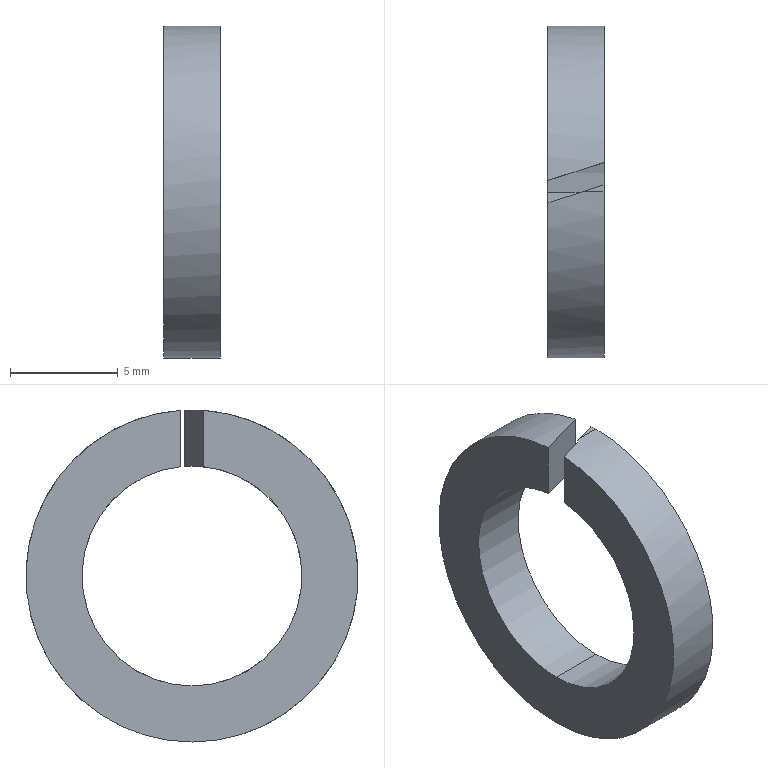Part | SolidWorks | features BaseBody 1 | 1 solid | 10 faces | box 2.6 x 15.4 x 15.4 mm | volume 264.776 mm3 | cylinder 6 | plane 4 | commonest cylinder face diameters 10.2 x3 15.4 x3
STEP:
#1=CARTESIAN_POINT('',(2.6,0.3248,7.693));
#2=VERTEX_POINT('',#1);
#3=CARTESIAN_POINT('',(1.6,0.,7.7));
#4=VERTEX_POINT('',#3);
#5=CARTESIAN_POINT('',(2.6,0.3248,7.693));
#6=CARTESIAN_POINT('',(2.267,0.2166,7.698));
#7=CARTESIAN_POINT('',(1.934,0.1083,7.7));
#8=CARTESIAN_POINT('',(1.6,0.,7.7));
#9=(BOUNDED_CURVE()B_SPLINE_CURVE(3,(#5,#6,#7,#8),.UNSPECIFIED.,.F.,.F.)B_SPLINE_CURVE_WITH_KNOTS((4,4),(1.529,1.571),.UNSPECIFIED.)CURVE()GEOMETRIC_REPRESENTATION_ITEM()RATIONAL_B_SPLINE_CURVE((1.,0.9999,0.9999,1.))REPRESENTATION_ITEM(''));
#10=EDGE_CURVE('',#2,#4,#9,.T.);
#11=ORIENTED_EDGE('',*,*,#10,.T.);
#12=CARTESIAN_POINT('',(2.6,0.,7.7));
#13=VERTEX_POINT('',#12);
#14=CARTESIAN_POINT('',(0.,0.,7.7));
#15=DIRECTION('',(1.,0.,0.));
#16=VECTOR('',#15,1000.);
#17=LINE('',#14,#16);
#18=EDGE_CURVE('',#4,#13,#17,.T.);
#19=ORIENTED_EDGE('',*,*,#18,.T.);
#20=CARTESIAN_POINT('',(2.6,0.,0.));
#21=DIRECTION('',(-1.,0.,0.));
#22=DIRECTION('',(0.,0.,-1.));
#23=AXIS2_PLACEMENT_3D('',#20,#21,#22);
#24=CIRCLE('',#23,7.7);
#25=EDGE_CURVE('',#13,#2,#24,.T.);
#26=ORIENTED_EDGE('',*,*,#25,.T.);
#27=EDGE_LOOP('',(#11,#19,#26));
#28=FACE_OUTER_BOUND('',#27,.T.);
#29=CARTESIAN_POINT('',(0.,0.,0.));
#30=DIRECTION('',(1.,0.,0.));
#31=DIRECTION('',(0.,0.,-1.));
#32=AXIS2_PLACEMENT_3D('',#29,#30,#31);
#33=CYLINDRICAL_SURFACE('',#32,7.7);
#34=ADVANCED_FACE('',(#28),#33,.T.);
#35=ORIENTED_EDGE('',*,*,#18,.F.);
#36=CARTESIAN_POINT('',(0.,-0.52,7.682));
#37=VERTEX_POINT('',#36);
#38=CARTESIAN_POINT('',(1.6,0.,7.7));
#39=CARTESIAN_POINT('',(1.066,-0.1735,7.7));
#40=CARTESIAN_POINT('',(0.5328,-0.3469,7.694));
#41=CARTESIAN_POINT('',(0.,-0.52,7.682));
#42=(BOUNDED_CURVE()B_SPLINE_CURVE(3,(#38,#39,#40,#41),.UNSPECIFIED.,.F.,.F.)B_SPLINE_CURVE_WITH_KNOTS((4,4),(1.571,1.638),.UNSPECIFIED.)CURVE()GEOMETRIC_REPRESENTATION_ITEM()RATIONAL_B_SPLINE_CURVE((1.,0.9996,0.9996,1.))REPRESENTATION_ITEM(''));
#43=EDGE_CURVE('',#4,#37,#42,.T.);
#44=ORIENTED_EDGE('',*,*,#43,.T.);
#45=CARTESIAN_POINT('',(0.,0.,-7.7));
#46=VERTEX_POINT('',#45);
#47=CARTESIAN_POINT('',(0.,0.,0.));
#48=DIRECTION('',(1.,0.,0.));
#49=DIRECTION('',(0.,0.,-1.));
#50=AXIS2_PLACEMENT_3D('',#47,#48,#49);
#51=CIRCLE('',#50,7.7);
#52=EDGE_CURVE('',#37,#46,#51,.T.);
#53=ORIENTED_EDGE('',*,*,#52,.T.);
#54=CARTESIAN_POINT('',(2.6,0.,-7.7));
#55=VERTEX_POINT('',#54);
#56=CARTESIAN_POINT('',(0.,0.,-7.7));
#57=DIRECTION('',(1.,0.,0.));
#58=VECTOR('',#57,1000.);
#59=LINE('',#56,#58);
#60=EDGE_CURVE('',#46,#55,#59,.T.);
#61=ORIENTED_EDGE('',*,*,#60,.T.);
#62=CARTESIAN_POINT('',(2.6,0.,0.));
#63=DIRECTION('',(-1.,0.,0.));
#64=DIRECTION('',(0.,0.,-1.));
#65=AXIS2_PLACEMENT_3D('',#62,#63,#64);
#66=CIRCLE('',#65,7.7);
#67=EDGE_CURVE('',#55,#13,#66,.T.);
#68=ORIENTED_EDGE('',*,*,#67,.T.);
#69=EDGE_LOOP('',(#35,#44,#53,#61,#68));
#70=FACE_OUTER_BOUND('',#69,.T.);
#71=CARTESIAN_POINT('',(0.,0.,0.));
#72=DIRECTION('',(1.,0.,0.));
#73=DIRECTION('',(0.,0.,-1.));
#74=AXIS2_PLACEMENT_3D('',#71,#72,#73);
#75=CYLINDRICAL_SURFACE('',#74,7.7);
#76=ADVANCED_FACE('',(#70),#75,.T.);
#77=CARTESIAN_POINT('',(0.,-0.52,5.073));
#78=VERTEX_POINT('',#77);
#79=CARTESIAN_POINT('',(1.6,0.,5.1));
#80=VERTEX_POINT('',#79);
#81=CARTESIAN_POINT('',(0.,-0.52,5.073));
#82=CARTESIAN_POINT('',(0.5318,-0.3472,5.091));
#83=CARTESIAN_POINT('',(1.066,-0.1737,5.1));
#84=CARTESIAN_POINT('',(1.6,0.,5.1));
#85=(BOUNDED_CURVE()B_SPLINE_CURVE(3,(#81,#82,#83,#84),.UNSPECIFIED.,.F.,.F.)B_SPLINE_CURVE_WITH_KNOTS((4,4),(4.61,4.712),.UNSPECIFIED.)CURVE()GEOMETRIC_REPRESENTATION_ITEM()RATIONAL_B_SPLINE_CURVE((1.,0.9991,0.9991,1.))REPRESENTATION_ITEM(''));
#86=EDGE_CURVE('',#78,#80,#85,.T.);
#87=ORIENTED_EDGE('',*,*,#86,.T.);
#88=CARTESIAN_POINT('',(2.6,0.,5.1));
#89=VERTEX_POINT('',#88);
#90=CARTESIAN_POINT('',(0.,0.,5.1));
#91=DIRECTION('',(1.,0.,0.));
#92=VECTOR('',#91,1000.);
#93=LINE('',#90,#92);
#94=EDGE_CURVE('',#80,#89,#93,.T.);
#95=ORIENTED_EDGE('',*,*,#94,.T.);
#96=CARTESIAN_POINT('',(2.6,0.,-5.1));
#97=VERTEX_POINT('',#96);
#98=CARTESIAN_POINT('',(2.6,0.,0.));
#99=DIRECTION('',(1.,0.,0.));
#100=DIRECTION('',(0.,0.,-1.));
#101=AXIS2_PLACEMENT_3D('',#98,#99,#100);
#102=CIRCLE('',#101,5.1);
#103=EDGE_CURVE('',#89,#97,#102,.T.);
#104=ORIENTED_EDGE('',*,*,#103,.T.);
#105=CARTESIAN_POINT('',(0.,0.,-5.1));
#106=VERTEX_POINT('',#105);
#107=CARTESIAN_POINT('',(0.,0.,-5.1));
#108=DIRECTION('',(1.,0.,0.));
#109=VECTOR('',#108,1000.);
#110=LINE('',#107,#109);
#111=EDGE_CURVE('',#106,#97,#110,.T.);
#112=ORIENTED_EDGE('',*,*,#111,.F.);
#113=CARTESIAN_POINT('',(0.,0.,0.));
#114=DIRECTION('',(1.,0.,0.));
#115=DIRECTION('',(0.,0.,-1.));
#116=AXIS2_PLACEMENT_3D('',#113,#114,#115);
#117=CIRCLE('',#116,5.1);
#118=EDGE_CURVE('',#78,#106,#117,.T.);
#119=ORIENTED_EDGE('',*,*,#118,.F.);
#120=EDGE_LOOP('',(#87,#95,#104,#112,#119));
#121=FACE_OUTER_BOUND('',#120,.T.);
#122=CARTESIAN_POINT('',(0.,0.,0.));
#123=DIRECTION('',(1.,0.,0.));
#124=DIRECTION('',(0.,0.,-1.));
#125=AXIS2_PLACEMENT_3D('',#122,#123,#124);
#126=CYLINDRICAL_SURFACE('',#125,5.1);
#127=ADVANCED_FACE('',(#121),#126,.F.);
#128=CARTESIAN_POINT('',(0.,0.52,5.073));
#129=VERTEX_POINT('',#128);
#130=CARTESIAN_POINT('',(0.,0.,0.));
#131=DIRECTION('',(1.,0.,0.));
#132=DIRECTION('',(0.,0.,-1.));
#133=AXIS2_PLACEMENT_3D('',#130,#131,#132);
#134=CIRCLE('',#133,5.1);
#135=EDGE_CURVE('',#106,#129,#134,.T.);
#136=ORIENTED_EDGE('',*,*,#135,.F.);
#137=ORIENTED_EDGE('',*,*,#111,.T.);
#138=CARTESIAN_POINT('',(2.6,1.365,4.914));
#139=VERTEX_POINT('',#138);
#140=CARTESIAN_POINT('',(2.6,0.,0.));
#141=DIRECTION('',(1.,0.,0.));
#142=DIRECTION('',(0.,0.,-1.));
#143=AXIS2_PLACEMENT_3D('',#140,#141,#142);
#144=CIRCLE('',#143,5.1);
#145=EDGE_CURVE('',#97,#139,#144,.T.);
#146=ORIENTED_EDGE('',*,*,#145,.T.);
#147=CARTESIAN_POINT('',(2.6,1.365,4.914));
#148=CARTESIAN_POINT('',(1.748,1.088,4.991));
#149=CARTESIAN_POINT('',(0.8795,0.8058,5.044));
#150=CARTESIAN_POINT('',(0.,0.52,5.073));
#151=(BOUNDED_CURVE()B_SPLINE_CURVE(3,(#147,#148,#149,#150),.UNSPECIFIED.,.F.,.F.)B_SPLINE_CURVE_WITH_KNOTS((4,4),(1.3,1.469),.UNSPECIFIED.)CURVE()GEOMETRIC_REPRESENTATION_ITEM()RATIONAL_B_SPLINE_CURVE((1.,0.9976,0.9976,1.))REPRESENTATION_ITEM(''));
#152=EDGE_CURVE('',#139,#129,#151,.T.);
#153=ORIENTED_EDGE('',*,*,#152,.T.);
#154=EDGE_LOOP('',(#136,#137,#146,#153));
#155=FACE_OUTER_BOUND('',#154,.T.);
#156=CARTESIAN_POINT('',(0.,0.,0.));
#157=DIRECTION('',(1.,0.,0.));
#158=DIRECTION('',(0.,0.,-1.));
#159=AXIS2_PLACEMENT_3D('',#156,#157,#158);
#160=CYLINDRICAL_SURFACE('',#159,5.1);
#161=ADVANCED_FACE('',(#155),#160,.F.);
#162=ORIENTED_EDGE('',*,*,#60,.F.);
#163=CARTESIAN_POINT('',(0.,0.52,7.682));
#164=VERTEX_POINT('',#163);
#165=CARTESIAN_POINT('',(0.,0.,0.));
#166=DIRECTION('',(1.,0.,0.));
#167=DIRECTION('',(0.,0.,-1.));
#168=AXIS2_PLACEMENT_3D('',#165,#166,#167);
#169=CIRCLE('',#168,7.7);
#170=EDGE_CURVE('',#46,#164,#169,.T.);
#171=ORIENTED_EDGE('',*,*,#170,.T.);
#172=CARTESIAN_POINT('',(2.6,1.365,7.578));
#173=VERTEX_POINT('',#172);
#174=CARTESIAN_POINT('',(0.,0.52,7.682));
#175=CARTESIAN_POINT('',(0.8721,0.8034,7.663));
#176=CARTESIAN_POINT('',(1.74,1.085,7.628));
#177=CARTESIAN_POINT('',(2.6,1.365,7.578));
#178=(BOUNDED_CURVE()B_SPLINE_CURVE(3,(#174,#175,#176,#177),.UNSPECIFIED.,.F.,.F.)B_SPLINE_CURVE_WITH_KNOTS((4,4),(4.78,4.891),.UNSPECIFIED.)CURVE()GEOMETRIC_REPRESENTATION_ITEM()RATIONAL_B_SPLINE_CURVE((1.,0.999,0.999,1.))REPRESENTATION_ITEM(''));
#179=EDGE_CURVE('',#164,#173,#178,.T.);
#180=ORIENTED_EDGE('',*,*,#179,.T.);
#181=CARTESIAN_POINT('',(2.6,0.,0.));
#182=DIRECTION('',(-1.,0.,0.));
#183=DIRECTION('',(0.,0.,-1.));
#184=AXIS2_PLACEMENT_3D('',#181,#182,#183);
#185=CIRCLE('',#184,7.7);
#186=EDGE_CURVE('',#173,#55,#185,.T.);
#187=ORIENTED_EDGE('',*,*,#186,.T.);
#188=EDGE_LOOP('',(#162,#171,#180,#187));
#189=FACE_OUTER_BOUND('',#188,.T.);
#190=CARTESIAN_POINT('',(0.,0.,0.));
#191=DIRECTION('',(1.,0.,0.));
#192=DIRECTION('',(0.,0.,-1.));
#193=AXIS2_PLACEMENT_3D('',#190,#191,#192);
#194=CYLINDRICAL_SURFACE('',#193,7.7);
#195=ADVANCED_FACE('',(#189),#194,.T.);
#196=ORIENTED_EDGE('',*,*,#186,.F.);
#197=CARTESIAN_POINT('',(2.6,1.365,0.));
#198=DIRECTION('',(0.,0.,1.));
#199=VECTOR('',#198,1000.);
#200=LINE('',#197,#199);
#201=EDGE_CURVE('',#139,#173,#200,.T.);
#202=ORIENTED_EDGE('',*,*,#201,.F.);
#203=ORIENTED_EDGE('',*,*,#145,.F.);
#204=ORIENTED_EDGE('',*,*,#103,.F.);
#205=CARTESIAN_POINT('',(2.6,0.3248,5.09));
#206=VERTEX_POINT('',#205);
#207=CARTESIAN_POINT('',(2.6,0.,0.));
#208=DIRECTION('',(1.,0.,0.));
#209=DIRECTION('',(0.,0.,-1.));
#210=AXIS2_PLACEMENT_3D('',#207,#208,#209);
#211=CIRCLE('',#210,5.1);
#212=EDGE_CURVE('',#206,#89,#211,.T.);
#213=ORIENTED_EDGE('',*,*,#212,.F.);
#214=CARTESIAN_POINT('',(2.6,0.3248,0.));
#215=DIRECTION('',(0.,0.,-1.));
#216=VECTOR('',#215,1000.);
#217=LINE('',#214,#216);
#218=EDGE_CURVE('',#2,#206,#217,.T.);
#219=ORIENTED_EDGE('',*,*,#218,.F.);
#220=ORIENTED_EDGE('',*,*,#25,.F.);
#221=ORIENTED_EDGE('',*,*,#67,.F.);
#222=EDGE_LOOP('',(#196,#202,#203,#204,#213,#219,#220,#221));
#223=FACE_OUTER_BOUND('',#222,.T.);
#224=CARTESIAN_POINT('',(2.6,0.,0.));
#225=DIRECTION('',(-1.,0.,0.));
#226=DIRECTION('',(0.,0.,1.));
#227=AXIS2_PLACEMENT_3D('',#224,#225,#226);
#228=PLANE('',#227);
#229=ADVANCED_FACE('',(#223),#228,.F.);
#230=ORIENTED_EDGE('',*,*,#201,.T.);
#231=ORIENTED_EDGE('',*,*,#179,.F.);
#232=CARTESIAN_POINT('',(0.,0.52,0.));
#233=DIRECTION('',(0.,0.,1.));
#234=VECTOR('',#233,1000.);
#235=LINE('',#232,#234);
#236=EDGE_CURVE('',#129,#164,#235,.T.);
#237=ORIENTED_EDGE('',*,*,#236,.F.);
#238=ORIENTED_EDGE('',*,*,#152,.F.);
#239=EDGE_LOOP('',(#230,#231,#237,#238));
#240=FACE_OUTER_BOUND('',#239,.T.);
#241=CARTESIAN_POINT('',(0.,0.52,0.));
#242=DIRECTION('',(-0.309,0.9511,0.));
#243=DIRECTION('',(-0.9511,-0.309,0.));
#244=AXIS2_PLACEMENT_3D('',#241,#242,#243);
#245=PLANE('',#244);
#246=ADVANCED_FACE('',(#240),#245,.F.);
#247=ORIENTED_EDGE('',*,*,#236,.T.);
#248=ORIENTED_EDGE('',*,*,#170,.F.);
#249=ORIENTED_EDGE('',*,*,#52,.F.);
#250=CARTESIAN_POINT('',(0.,-0.52,0.));
#251=DIRECTION('',(0.,0.,-1.));
#252=VECTOR('',#251,1000.);
#253=LINE('',#250,#252);
#254=EDGE_CURVE('',#37,#78,#253,.T.);
#255=ORIENTED_EDGE('',*,*,#254,.T.);
#256=ORIENTED_EDGE('',*,*,#118,.T.);
#257=ORIENTED_EDGE('',*,*,#135,.T.);
#258=EDGE_LOOP('',(#247,#248,#249,#255,#256,#257));
#259=FACE_OUTER_BOUND('',#258,.T.);
#260=CARTESIAN_POINT('',(0.,0.,0.));
#261=DIRECTION('',(-1.,0.,0.));
#262=DIRECTION('',(0.,0.,1.));
#263=AXIS2_PLACEMENT_3D('',#260,#261,#262);
#264=PLANE('',#263);
#265=ADVANCED_FACE('',(#259),#264,.T.);
#266=ORIENTED_EDGE('',*,*,#254,.F.);
#267=ORIENTED_EDGE('',*,*,#43,.F.);
#268=ORIENTED_EDGE('',*,*,#10,.F.);
#269=ORIENTED_EDGE('',*,*,#218,.T.);
#270=CARTESIAN_POINT('',(1.6,0.,5.1));
#271=CARTESIAN_POINT('',(1.934,0.1084,5.1));
#272=CARTESIAN_POINT('',(2.267,0.2167,5.097));
#273=CARTESIAN_POINT('',(2.6,0.3248,5.09));
#274=(BOUNDED_CURVE()B_SPLINE_CURVE(3,(#270,#271,#272,#273),.UNSPECIFIED.,.F.,.F.)B_SPLINE_CURVE_WITH_KNOTS((4,4),(4.712,4.776),.UNSPECIFIED.)CURVE()GEOMETRIC_REPRESENTATION_ITEM()RATIONAL_B_SPLINE_CURVE((1.,0.9997,0.9997,1.))REPRESENTATION_ITEM(''));
#275=EDGE_CURVE('',#80,#206,#274,.T.);
#276=ORIENTED_EDGE('',*,*,#275,.F.);
#277=ORIENTED_EDGE('',*,*,#86,.F.);
#278=EDGE_LOOP('',(#266,#267,#268,#269,#276,#277));
#279=FACE_OUTER_BOUND('',#278,.T.);
#280=CARTESIAN_POINT('',(2.6,0.3248,0.));
#281=DIRECTION('',(0.309,-0.9511,0.));
#282=DIRECTION('',(0.9511,0.309,0.));
#283=AXIS2_PLACEMENT_3D('',#280,#281,#282);
#284=PLANE('',#283);
#285=ADVANCED_FACE('',(#279),#284,.F.);
#286=ORIENTED_EDGE('',*,*,#94,.F.);
#287=ORIENTED_EDGE('',*,*,#275,.T.);
#288=ORIENTED_EDGE('',*,*,#212,.T.);
#289=EDGE_LOOP('',(#286,#287,#288));
#290=FACE_OUTER_BOUND('',#289,.T.);
#291=CARTESIAN_POINT('',(0.,0.,0.));
#292=DIRECTION('',(1.,0.,0.));
#293=DIRECTION('',(0.,0.,-1.));
#294=AXIS2_PLACEMENT_3D('',#291,#292,#293);
#295=CYLINDRICAL_SURFACE('',#294,5.1);
#296=ADVANCED_FACE('',(#290),#295,.F.);
#297=CLOSED_SHELL('',(#34,#76,#127,#161,#195,#229,#246,#265,#285,#296));
#298=MANIFOLD_SOLID_BREP('',#297);
#299=CARTESIAN_POINT('',(0.,0.,0.));
#300=DIRECTION('',(0.,0.,1.));
#301=DIRECTION('',(1.,0.,0.));
#302=AXIS2_PLACEMENT_3D('',#299,#300,#301);
#303=(LENGTH_UNIT()NAMED_UNIT(*)SI_UNIT(.MILLI.,.METRE.));
#304=UNCERTAINTY_MEASURE_WITH_UNIT(LENGTH_MEASURE(0.00001),#303,'','');
#305=(NAMED_UNIT(*)PLANE_ANGLE_UNIT()SI_UNIT($,.RADIAN.));
#306=(NAMED_UNIT(*)SI_UNIT($,.STERADIAN.)SOLID_ANGLE_UNIT());
#307=(GEOMETRIC_REPRESENTATION_CONTEXT(3)GLOBAL_UNCERTAINTY_ASSIGNED_CONTEXT((#304))GLOBAL_UNIT_ASSIGNED_CONTEXT((#303,#305,#306))REPRESENTATION_CONTEXT('',''));
#308=ADVANCED_BREP_SHAPE_REPRESENTATION('',(#298,#302),#307);